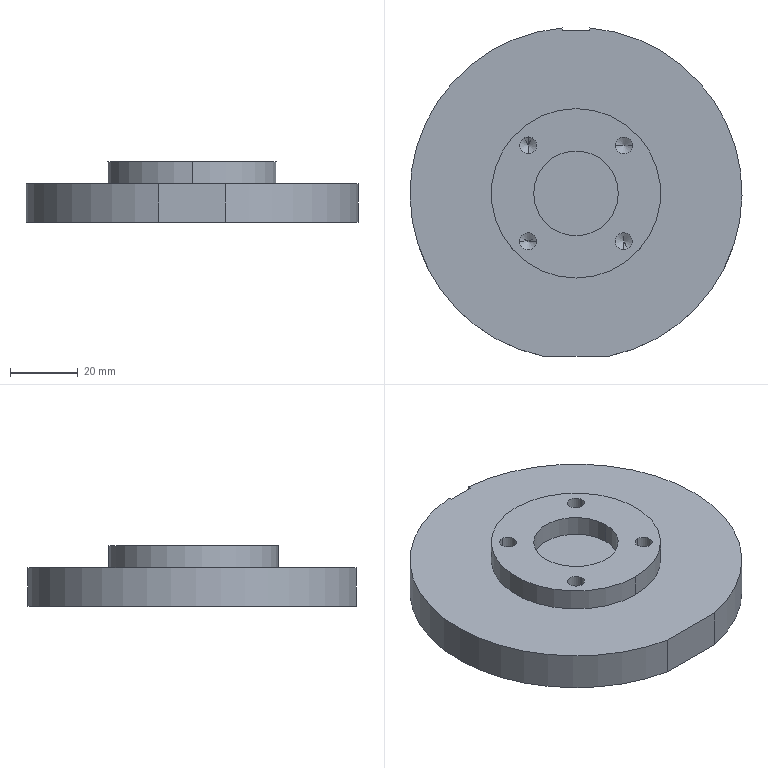Part | STEP file | Link6 | 1 solid | 30 faces | box 98 x 96.836 x 18 mm | volume 95263 mm3 | cylinder 14 | cone 8 | plane 8 | commonest cylinder face diameters 5 x8 25 x2 50 x2 98 x2
STEP:
#1=CARTESIAN_POINT('',(-12.5,0.,-6.));
#2=VERTEX_POINT('',#1);
#3=CARTESIAN_POINT('',(12.5,0.,-6.));
#4=VERTEX_POINT('',#3);
#5=CARTESIAN_POINT('',(0.,0.,-6.));
#6=DIRECTION('',(0.,0.,1.));
#7=DIRECTION('',(1.,0.,0.));
#8=AXIS2_PLACEMENT_3D('',#5,#6,#7);
#9=CIRCLE('',#8,12.5);
#10=EDGE_CURVE('',#2,#4,#9,.T.);
#11=ORIENTED_EDGE('',*,*,#10,.F.);
#12=CARTESIAN_POINT('',(-12.5,0.,0.));
#13=VERTEX_POINT('',#12);
#14=CARTESIAN_POINT('',(-12.5,0.,-6.));
#15=DIRECTION('',(0.,0.,1.));
#16=VECTOR('',#15,1000.);
#17=LINE('',#14,#16);
#18=EDGE_CURVE('',#2,#13,#17,.T.);
#19=ORIENTED_EDGE('',*,*,#18,.T.);
#20=CARTESIAN_POINT('',(12.5,0.,0.));
#21=VERTEX_POINT('',#20);
#22=CARTESIAN_POINT('',(0.,0.,0.));
#23=DIRECTION('',(0.,0.,1.));
#24=DIRECTION('',(1.,0.,0.));
#25=AXIS2_PLACEMENT_3D('',#22,#23,#24);
#26=CIRCLE('',#25,12.5);
#27=EDGE_CURVE('',#13,#21,#26,.T.);
#28=ORIENTED_EDGE('',*,*,#27,.T.);
#29=CARTESIAN_POINT('',(12.5,0.,-6.));
#30=DIRECTION('',(0.,0.,1.));
#31=VECTOR('',#30,1000.);
#32=LINE('',#29,#31);
#33=EDGE_CURVE('',#4,#21,#32,.T.);
#34=ORIENTED_EDGE('',*,*,#33,.F.);
#35=EDGE_LOOP('',(#11,#19,#28,#34));
#36=FACE_OUTER_BOUND('',#35,.T.);
#37=CARTESIAN_POINT('',(0.,0.,-6.));
#38=DIRECTION('',(0.,0.,1.));
#39=DIRECTION('',(1.,0.,0.));
#40=AXIS2_PLACEMENT_3D('',#37,#38,#39);
#41=CYLINDRICAL_SURFACE('',#40,12.5);
#42=ADVANCED_FACE('',(#36),#41,.F.);
#43=CARTESIAN_POINT('',(-14.142,11.642,-13.));
#44=VERTEX_POINT('',#43);
#45=CARTESIAN_POINT('',(-14.142,16.642,-13.));
#46=VERTEX_POINT('',#45);
#47=CARTESIAN_POINT('',(-14.142,14.142,-13.));
#48=DIRECTION('',(0.,0.,1.));
#49=DIRECTION('',(0.,1.,0.));
#50=AXIS2_PLACEMENT_3D('',#47,#48,#49);
#51=CIRCLE('',#50,2.5);
#52=EDGE_CURVE('',#44,#46,#51,.T.);
#53=ORIENTED_EDGE('',*,*,#52,.F.);
#54=CARTESIAN_POINT('',(-14.142,11.642,0.));
#55=VERTEX_POINT('',#54);
#56=CARTESIAN_POINT('',(-14.142,11.642,0.));
#57=DIRECTION('',(0.,0.,1.));
#58=VECTOR('',#57,1000.);
#59=LINE('',#56,#58);
#60=EDGE_CURVE('',#44,#55,#59,.T.);
#61=ORIENTED_EDGE('',*,*,#60,.T.);
#62=CARTESIAN_POINT('',(-14.142,16.642,0.));
#63=VERTEX_POINT('',#62);
#64=CARTESIAN_POINT('',(-14.142,14.142,0.));
#65=DIRECTION('',(0.,0.,1.));
#66=DIRECTION('',(0.,1.,0.));
#67=AXIS2_PLACEMENT_3D('',#64,#65,#66);
#68=CIRCLE('',#67,2.5);
#69=EDGE_CURVE('',#55,#63,#68,.T.);
#70=ORIENTED_EDGE('',*,*,#69,.T.);
#71=CARTESIAN_POINT('',(-14.142,16.642,0.));
#72=DIRECTION('',(0.,0.,1.));
#73=VECTOR('',#72,1000.);
#74=LINE('',#71,#73);
#75=EDGE_CURVE('',#46,#63,#74,.T.);
#76=ORIENTED_EDGE('',*,*,#75,.F.);
#77=EDGE_LOOP('',(#53,#61,#70,#76));
#78=FACE_OUTER_BOUND('',#77,.T.);
#79=CARTESIAN_POINT('',(-14.142,14.142,0.));
#80=DIRECTION('',(0.,0.,1.));
#81=DIRECTION('',(0.,1.,0.));
#82=AXIS2_PLACEMENT_3D('',#79,#80,#81);
#83=CYLINDRICAL_SURFACE('',#82,2.5);
#84=ADVANCED_FACE('',(#78),#83,.F.);
#85=CARTESIAN_POINT('',(-14.142,14.142,-14.502));
#86=VERTEX_POINT('',#85);
#87=CARTESIAN_POINT('',(-14.142,16.642,-13.));
#88=DIRECTION('',(0.,0.8572,0.515));
#89=VECTOR('',#88,1000.);
#90=LINE('',#87,#89);
#91=EDGE_CURVE('',#86,#46,#90,.T.);
#92=ORIENTED_EDGE('',*,*,#91,.F.);
#93=CARTESIAN_POINT('',(-14.142,11.642,-13.));
#94=DIRECTION('',(0.,-0.8572,0.515));
#95=VECTOR('',#94,1000.);
#96=LINE('',#93,#95);
#97=EDGE_CURVE('',#86,#44,#96,.T.);
#98=ORIENTED_EDGE('',*,*,#97,.T.);
#99=ORIENTED_EDGE('',*,*,#52,.T.);
#100=EDGE_LOOP('',(#92,#98,#99));
#101=FACE_OUTER_BOUND('',#100,.T.);
#102=CARTESIAN_POINT('',(-14.142,14.142,-13.));
#103=DIRECTION('',(0.,0.,1.));
#104=DIRECTION('',(0.,1.,0.));
#105=AXIS2_PLACEMENT_3D('',#102,#103,#104);
#106=CONICAL_SURFACE('',#105,2.5,1.03);
#107=ADVANCED_FACE('',(#101),#106,.F.);
#108=CARTESIAN_POINT('',(-11.642,-14.142,-13.));
#109=VERTEX_POINT('',#108);
#110=CARTESIAN_POINT('',(-16.642,-14.142,-13.));
#111=VERTEX_POINT('',#110);
#112=CARTESIAN_POINT('',(-14.142,-14.142,-13.));
#113=DIRECTION('',(0.,0.,1.));
#114=DIRECTION('',(-1.,0.,0.));
#115=AXIS2_PLACEMENT_3D('',#112,#113,#114);
#116=CIRCLE('',#115,2.5);
#117=EDGE_CURVE('',#109,#111,#116,.T.);
#118=ORIENTED_EDGE('',*,*,#117,.F.);
#119=CARTESIAN_POINT('',(-11.642,-14.142,0.));
#120=VERTEX_POINT('',#119);
#121=CARTESIAN_POINT('',(-11.642,-14.142,0.));
#122=DIRECTION('',(0.,0.,1.));
#123=VECTOR('',#122,1000.);
#124=LINE('',#121,#123);
#125=EDGE_CURVE('',#109,#120,#124,.T.);
#126=ORIENTED_EDGE('',*,*,#125,.T.);
#127=CARTESIAN_POINT('',(-16.642,-14.142,0.));
#128=VERTEX_POINT('',#127);
#129=CARTESIAN_POINT('',(-14.142,-14.142,0.));
#130=DIRECTION('',(0.,0.,1.));
#131=DIRECTION('',(-1.,0.,0.));
#132=AXIS2_PLACEMENT_3D('',#129,#130,#131);
#133=CIRCLE('',#132,2.5);
#134=EDGE_CURVE('',#120,#128,#133,.T.);
#135=ORIENTED_EDGE('',*,*,#134,.T.);
#136=CARTESIAN_POINT('',(-16.642,-14.142,0.));
#137=DIRECTION('',(0.,0.,1.));
#138=VECTOR('',#137,1000.);
#139=LINE('',#136,#138);
#140=EDGE_CURVE('',#111,#128,#139,.T.);
#141=ORIENTED_EDGE('',*,*,#140,.F.);
#142=EDGE_LOOP('',(#118,#126,#135,#141));
#143=FACE_OUTER_BOUND('',#142,.T.);
#144=CARTESIAN_POINT('',(-14.142,-14.142,0.));
#145=DIRECTION('',(0.,0.,1.));
#146=DIRECTION('',(-1.,0.,0.));
#147=AXIS2_PLACEMENT_3D('',#144,#145,#146);
#148=CYLINDRICAL_SURFACE('',#147,2.5);
#149=ADVANCED_FACE('',(#143),#148,.F.);
#150=CARTESIAN_POINT('',(-14.142,-14.142,-14.502));
#151=VERTEX_POINT('',#150);
#152=CARTESIAN_POINT('',(-16.642,-14.142,-13.));
#153=DIRECTION('',(-0.8572,0.,0.515));
#154=VECTOR('',#153,1000.);
#155=LINE('',#152,#154);
#156=EDGE_CURVE('',#151,#111,#155,.T.);
#157=ORIENTED_EDGE('',*,*,#156,.F.);
#158=CARTESIAN_POINT('',(-11.642,-14.142,-13.));
#159=DIRECTION('',(0.8572,0.,0.515));
#160=VECTOR('',#159,1000.);
#161=LINE('',#158,#160);
#162=EDGE_CURVE('',#151,#109,#161,.T.);
#163=ORIENTED_EDGE('',*,*,#162,.T.);
#164=ORIENTED_EDGE('',*,*,#117,.T.);
#165=EDGE_LOOP('',(#157,#163,#164));
#166=FACE_OUTER_BOUND('',#165,.T.);
#167=CARTESIAN_POINT('',(-14.142,-14.142,-13.));
#168=DIRECTION('',(0.,0.,1.));
#169=DIRECTION('',(-1.,0.,0.));
#170=AXIS2_PLACEMENT_3D('',#167,#168,#169);
#171=CONICAL_SURFACE('',#170,2.5,1.03);
#172=ADVANCED_FACE('',(#166),#171,.F.);
#173=CARTESIAN_POINT('',(14.142,-11.642,-13.));
#174=VERTEX_POINT('',#173);
#175=CARTESIAN_POINT('',(14.142,-16.642,-13.));
#176=VERTEX_POINT('',#175);
#177=CARTESIAN_POINT('',(14.142,-14.142,-13.));
#178=DIRECTION('',(0.,0.,1.));
#179=DIRECTION('',(0.,-1.,0.));
#180=AXIS2_PLACEMENT_3D('',#177,#178,#179);
#181=CIRCLE('',#180,2.5);
#182=EDGE_CURVE('',#174,#176,#181,.T.);
#183=ORIENTED_EDGE('',*,*,#182,.F.);
#184=CARTESIAN_POINT('',(14.142,-11.642,0.));
#185=VERTEX_POINT('',#184);
#186=CARTESIAN_POINT('',(14.142,-11.642,0.));
#187=DIRECTION('',(0.,0.,1.));
#188=VECTOR('',#187,1000.);
#189=LINE('',#186,#188);
#190=EDGE_CURVE('',#174,#185,#189,.T.);
#191=ORIENTED_EDGE('',*,*,#190,.T.);
#192=CARTESIAN_POINT('',(14.142,-16.642,0.));
#193=VERTEX_POINT('',#192);
#194=CARTESIAN_POINT('',(14.142,-14.142,0.));
#195=DIRECTION('',(0.,0.,1.));
#196=DIRECTION('',(0.,-1.,0.));
#197=AXIS2_PLACEMENT_3D('',#194,#195,#196);
#198=CIRCLE('',#197,2.5);
#199=EDGE_CURVE('',#185,#193,#198,.T.);
#200=ORIENTED_EDGE('',*,*,#199,.T.);
#201=CARTESIAN_POINT('',(14.142,-16.642,0.));
#202=DIRECTION('',(0.,0.,1.));
#203=VECTOR('',#202,1000.);
#204=LINE('',#201,#203);
#205=EDGE_CURVE('',#176,#193,#204,.T.);
#206=ORIENTED_EDGE('',*,*,#205,.F.);
#207=EDGE_LOOP('',(#183,#191,#200,#206));
#208=FACE_OUTER_BOUND('',#207,.T.);
#209=CARTESIAN_POINT('',(14.142,-14.142,0.));
#210=DIRECTION('',(0.,0.,1.));
#211=DIRECTION('',(0.,-1.,0.));
#212=AXIS2_PLACEMENT_3D('',#209,#210,#211);
#213=CYLINDRICAL_SURFACE('',#212,2.5);
#214=ADVANCED_FACE('',(#208),#213,.F.);
#215=CARTESIAN_POINT('',(14.142,-14.142,-14.502));
#216=VERTEX_POINT('',#215);
#217=CARTESIAN_POINT('',(14.142,-16.642,-13.));
#218=DIRECTION('',(0.,-0.8572,0.515));
#219=VECTOR('',#218,1000.);
#220=LINE('',#217,#219);
#221=EDGE_CURVE('',#216,#176,#220,.T.);
#222=ORIENTED_EDGE('',*,*,#221,.F.);
#223=CARTESIAN_POINT('',(14.142,-11.642,-13.));
#224=DIRECTION('',(0.,0.8572,0.515));
#225=VECTOR('',#224,1000.);
#226=LINE('',#223,#225);
#227=EDGE_CURVE('',#216,#174,#226,.T.);
#228=ORIENTED_EDGE('',*,*,#227,.T.);
#229=ORIENTED_EDGE('',*,*,#182,.T.);
#230=EDGE_LOOP('',(#222,#228,#229));
#231=FACE_OUTER_BOUND('',#230,.T.);
#232=CARTESIAN_POINT('',(14.142,-14.142,-13.));
#233=DIRECTION('',(0.,0.,1.));
#234=DIRECTION('',(0.,-1.,0.));
#235=AXIS2_PLACEMENT_3D('',#232,#233,#234);
#236=CONICAL_SURFACE('',#235,2.5,1.03);
#237=ADVANCED_FACE('',(#231),#236,.F.);
#238=CARTESIAN_POINT('',(11.642,14.142,-13.));
#239=VERTEX_POINT('',#238);
#240=CARTESIAN_POINT('',(16.642,14.142,-13.));
#241=VERTEX_POINT('',#240);
#242=CARTESIAN_POINT('',(14.142,14.142,-13.));
#243=DIRECTION('',(0.,0.,1.));
#244=DIRECTION('',(1.,0.,0.));
#245=AXIS2_PLACEMENT_3D('',#242,#243,#244);
#246=CIRCLE('',#245,2.5);
#247=EDGE_CURVE('',#239,#241,#246,.T.);
#248=ORIENTED_EDGE('',*,*,#247,.F.);
#249=CARTESIAN_POINT('',(11.642,14.142,0.));
#250=VERTEX_POINT('',#249);
#251=CARTESIAN_POINT('',(11.642,14.142,0.));
#252=DIRECTION('',(0.,0.,1.));
#253=VECTOR('',#252,1000.);
#254=LINE('',#251,#253);
#255=EDGE_CURVE('',#239,#250,#254,.T.);
#256=ORIENTED_EDGE('',*,*,#255,.T.);
#257=CARTESIAN_POINT('',(16.642,14.142,0.));
#258=VERTEX_POINT('',#257);
#259=CARTESIAN_POINT('',(14.142,14.142,0.));
#260=DIRECTION('',(0.,0.,1.));
#261=DIRECTION('',(1.,0.,0.));
#262=AXIS2_PLACEMENT_3D('',#259,#260,#261);
#263=CIRCLE('',#262,2.5);
#264=EDGE_CURVE('',#250,#258,#263,.T.);
#265=ORIENTED_EDGE('',*,*,#264,.T.);
#266=CARTESIAN_POINT('',(16.642,14.142,0.));
#267=DIRECTION('',(0.,0.,1.));
#268=VECTOR('',#267,1000.);
#269=LINE('',#266,#268);
#270=EDGE_CURVE('',#241,#258,#269,.T.);
#271=ORIENTED_EDGE('',*,*,#270,.F.);
#272=EDGE_LOOP('',(#248,#256,#265,#271));
#273=FACE_OUTER_BOUND('',#272,.T.);
#274=CARTESIAN_POINT('',(14.142,14.142,0.));
#275=DIRECTION('',(0.,0.,1.));
#276=DIRECTION('',(1.,0.,0.));
#277=AXIS2_PLACEMENT_3D('',#274,#275,#276);
#278=CYLINDRICAL_SURFACE('',#277,2.5);
#279=ADVANCED_FACE('',(#273),#278,.F.);
#280=CARTESIAN_POINT('',(14.142,14.142,-14.502));
#281=VERTEX_POINT('',#280);
#282=CARTESIAN_POINT('',(16.642,14.142,-13.));
#283=DIRECTION('',(0.8572,0.,0.515));
#284=VECTOR('',#283,1000.);
#285=LINE('',#282,#284);
#286=EDGE_CURVE('',#281,#241,#285,.T.);
#287=ORIENTED_EDGE('',*,*,#286,.F.);
#288=CARTESIAN_POINT('',(11.642,14.142,-13.));
#289=DIRECTION('',(-0.8572,0.,0.515));
#290=VECTOR('',#289,1000.);
#291=LINE('',#288,#290);
#292=EDGE_CURVE('',#281,#239,#291,.T.);
#293=ORIENTED_EDGE('',*,*,#292,.T.);
#294=ORIENTED_EDGE('',*,*,#247,.T.);
#295=EDGE_LOOP('',(#287,#293,#294));
#296=FACE_OUTER_BOUND('',#295,.T.);
#297=CARTESIAN_POINT('',(14.142,14.142,-13.));
#298=DIRECTION('',(0.,0.,1.));
#299=DIRECTION('',(1.,0.,0.));
#300=AXIS2_PLACEMENT_3D('',#297,#298,#299);
#301=CONICAL_SURFACE('',#300,2.5,1.03);
#302=ADVANCED_FACE('',(#296),#301,.F.);
#303=CARTESIAN_POINT('',(0.,25.,0.));
#304=VERTEX_POINT('',#303);
#305=CARTESIAN_POINT('',(0.,-25.,0.));
#306=VERTEX_POINT('',#305);
#307=CARTESIAN_POINT('',(0.,0.,0.));
#308=DIRECTION('',(0.,0.,-1.));
#309=DIRECTION('',(0.,1.,0.));
#310=AXIS2_PLACEMENT_3D('',#307,#308,#309);
#311=CIRCLE('',#310,25.);
#312=EDGE_CURVE('',#304,#306,#311,.T.);
#313=ORIENTED_EDGE('',*,*,#312,.T.);
#314=CARTESIAN_POINT('',(0.,-25.,-6.5));
#315=VERTEX_POINT('',#314);
#316=CARTESIAN_POINT('',(0.,-25.,-3.25));
#317=DIRECTION('',(0.,0.,-1.));
#318=VECTOR('',#317,1000.);
#319=LINE('',#316,#318);
#320=EDGE_CURVE('',#306,#315,#319,.T.);
#321=ORIENTED_EDGE('',*,*,#320,.T.);
#322=CARTESIAN_POINT('',(0.,25.,-6.5));
#323=VERTEX_POINT('',#322);
#324=CARTESIAN_POINT('',(0.,0.,-6.5));
#325=DIRECTION('',(0.,0.,-1.));
#326=DIRECTION('',(0.,1.,0.));
#327=AXIS2_PLACEMENT_3D('',#324,#325,#326);
#328=CIRCLE('',#327,25.);
#329=EDGE_CURVE('',#323,#315,#328,.T.);
#330=ORIENTED_EDGE('',*,*,#329,.F.);
#331=CARTESIAN_POINT('',(0.,25.,-3.25));
#332=DIRECTION('',(0.,0.,-1.));
#333=VECTOR('',#332,1000.);
#334=LINE('',#331,#333);
#335=EDGE_CURVE('',#304,#323,#334,.T.);
#336=ORIENTED_EDGE('',*,*,#335,.F.);
#337=EDGE_LOOP('',(#313,#321,#330,#336));
#338=FACE_OUTER_BOUND('',#337,.T.);
#339=CARTESIAN_POINT('',(0.,0.,-3.25));
#340=DIRECTION('',(0.,0.,-1.));
#341=DIRECTION('',(0.,1.,0.));
#342=AXIS2_PLACEMENT_3D('',#339,#340,#341);
#343=CYLINDRICAL_SURFACE('',#342,25.);
#344=ADVANCED_FACE('',(#338),#343,.T.);
#345=CARTESIAN_POINT('',(4.,48.,-18.));
#346=VERTEX_POINT('',#345);
#347=CARTESIAN_POINT('',(4.,48.836,-18.));
#348=VERTEX_POINT('',#347);
#349=CARTESIAN_POINT('',(4.,48.836,-18.));
#350=DIRECTION('',(0.,1.,0.));
#351=VECTOR('',#350,1000.);
#352=LINE('',#349,#351);
#353=EDGE_CURVE('',#346,#348,#352,.T.);
#354=ORIENTED_EDGE('',*,*,#353,.T.);
#355=CARTESIAN_POINT('',(9.849,-48.,-18.));
#356=VERTEX_POINT('',#355);
#357=CARTESIAN_POINT('',(0.,0.,-18.));
#358=DIRECTION('',(0.,0.,-1.));
#359=DIRECTION('',(0.,1.,0.));
#360=AXIS2_PLACEMENT_3D('',#357,#358,#359);
#361=CIRCLE('',#360,49.);
#362=EDGE_CURVE('',#348,#356,#361,.T.);
#363=ORIENTED_EDGE('',*,*,#362,.T.);
#364=CARTESIAN_POINT('',(-9.849,-48.,-18.));
#365=VERTEX_POINT('',#364);
#366=CARTESIAN_POINT('',(0.,-48.,-18.));
#367=DIRECTION('',(-1.,0.,0.));
#368=VECTOR('',#367,1000.);
#369=LINE('',#366,#368);
#370=EDGE_CURVE('',#356,#365,#369,.T.);
#371=ORIENTED_EDGE('',*,*,#370,.T.);
#372=CARTESIAN_POINT('',(-4.,48.836,-18.));
#373=VERTEX_POINT('',#372);
#374=CARTESIAN_POINT('',(0.,0.,-18.));
#375=DIRECTION('',(0.,0.,-1.));
#376=DIRECTION('',(0.,1.,0.));
#377=AXIS2_PLACEMENT_3D('',#374,#375,#376);
#378=CIRCLE('',#377,49.);
#379=EDGE_CURVE('',#365,#373,#378,.T.);
#380=ORIENTED_EDGE('',*,*,#379,.T.);
#381=CARTESIAN_POINT('',(-4.,48.,-18.));
#382=VERTEX_POINT('',#381);
#383=CARTESIAN_POINT('',(-4.,48.,-18.));
#384=DIRECTION('',(0.,-1.,0.));
#385=VECTOR('',#384,1000.);
#386=LINE('',#383,#385);
#387=EDGE_CURVE('',#373,#382,#386,.T.);
#388=ORIENTED_EDGE('',*,*,#387,.T.);
#389=CARTESIAN_POINT('',(0.,48.,-18.));
#390=DIRECTION('',(1.,0.,0.));
#391=VECTOR('',#390,1000.);
#392=LINE('',#389,#391);
#393=EDGE_CURVE('',#382,#346,#392,.T.);
#394=ORIENTED_EDGE('',*,*,#393,.T.);
#395=EDGE_LOOP('',(#354,#363,#371,#380,#388,#394));
#396=FACE_OUTER_BOUND('',#395,.T.);
#397=CARTESIAN_POINT('',(0.,24.5,-18.));
#398=DIRECTION('',(0.,0.,-1.));
#399=DIRECTION('',(-1.,0.,0.));
#400=AXIS2_PLACEMENT_3D('',#397,#398,#399);
#401=PLANE('',#400);
#402=ADVANCED_FACE('',(#396),#401,.T.);
#403=CARTESIAN_POINT('',(4.,48.836,-6.5));
#404=VERTEX_POINT('',#403);
#405=CARTESIAN_POINT('',(4.,48.836,-12.25));
#406=DIRECTION('',(0.,0.,1.));
#407=VECTOR('',#406,1000.);
#408=LINE('',#405,#407);
#409=EDGE_CURVE('',#348,#404,#408,.T.);
#410=ORIENTED_EDGE('',*,*,#409,.T.);
#411=CARTESIAN_POINT('',(9.849,-48.,-6.5));
#412=VERTEX_POINT('',#411);
#413=CARTESIAN_POINT('',(0.,0.,-6.5));
#414=DIRECTION('',(0.,0.,-1.));
#415=DIRECTION('',(0.,1.,0.));
#416=AXIS2_PLACEMENT_3D('',#413,#414,#415);
#417=CIRCLE('',#416,49.);
#418=EDGE_CURVE('',#404,#412,#417,.T.);
#419=ORIENTED_EDGE('',*,*,#418,.T.);
#420=CARTESIAN_POINT('',(9.849,-48.,-12.25));
#421=DIRECTION('',(0.,0.,-1.));
#422=VECTOR('',#421,1000.);
#423=LINE('',#420,#422);
#424=EDGE_CURVE('',#412,#356,#423,.T.);
#425=ORIENTED_EDGE('',*,*,#424,.T.);
#426=ORIENTED_EDGE('',*,*,#362,.F.);
#427=EDGE_LOOP('',(#410,#419,#425,#426));
#428=FACE_OUTER_BOUND('',#427,.T.);
#429=CARTESIAN_POINT('',(0.,0.,-12.25));
#430=DIRECTION('',(0.,0.,-1.));
#431=DIRECTION('',(0.,1.,0.));
#432=AXIS2_PLACEMENT_3D('',#429,#430,#431);
#433=CYLINDRICAL_SURFACE('',#432,49.);
#434=ADVANCED_FACE('',(#428),#433,.T.);
#435=CARTESIAN_POINT('',(4.,48.,-6.5));
#436=VERTEX_POINT('',#435);
#437=CARTESIAN_POINT('',(4.,48.,-18.));
#438=DIRECTION('',(0.,0.,1.));
#439=VECTOR('',#438,1000.);
#440=LINE('',#437,#439);
#441=EDGE_CURVE('',#346,#436,#440,.T.);
#442=ORIENTED_EDGE('',*,*,#441,.F.);
#443=ORIENTED_EDGE('',*,*,#393,.F.);
#444=CARTESIAN_POINT('',(-4.,48.,-6.5));
#445=VERTEX_POINT('',#444);
#446=CARTESIAN_POINT('',(-4.,48.,-18.));
#447=DIRECTION('',(0.,0.,-1.));
#448=VECTOR('',#447,1000.);
#449=LINE('',#446,#448);
#450=EDGE_CURVE('',#445,#382,#449,.T.);
#451=ORIENTED_EDGE('',*,*,#450,.F.);
#452=CARTESIAN_POINT('',(4.,48.,-6.5));
#453=DIRECTION('',(-1.,0.,0.));
#454=VECTOR('',#453,1000.);
#455=LINE('',#452,#454);
#456=EDGE_CURVE('',#436,#445,#455,.T.);
#457=ORIENTED_EDGE('',*,*,#456,.F.);
#458=EDGE_LOOP('',(#442,#443,#451,#457));
#459=FACE_OUTER_BOUND('',#458,.T.);
#460=CARTESIAN_POINT('',(4.,48.,-18.));
#461=DIRECTION('',(0.,-1.,0.));
#462=DIRECTION('',(0.,0.,-1.));
#463=AXIS2_PLACEMENT_3D('',#460,#461,#462);
#464=PLANE('',#463);
#465=ADVANCED_FACE('',(#459),#464,.F.);
#466=CARTESIAN_POINT('',(-4.,48.836,-6.5));
#467=VERTEX_POINT('',#466);
#468=CARTESIAN_POINT('',(-4.,48.836,-12.25));
#469=DIRECTION('',(0.,0.,-1.));
#470=VECTOR('',#469,1000.);
#471=LINE('',#468,#470);
#472=EDGE_CURVE('',#467,#373,#471,.T.);
#473=ORIENTED_EDGE('',*,*,#472,.T.);
#474=ORIENTED_EDGE('',*,*,#379,.F.);
#475=CARTESIAN_POINT('',(-9.849,-48.,-6.5));
#476=VERTEX_POINT('',#475);
#477=CARTESIAN_POINT('',(-9.849,-48.,-12.25));
#478=DIRECTION('',(0.,0.,1.));
#479=VECTOR('',#478,1000.);
#480=LINE('',#477,#479);
#481=EDGE_CURVE('',#365,#476,#480,.T.);
#482=ORIENTED_EDGE('',*,*,#481,.T.);
#483=CARTESIAN_POINT('',(0.,0.,-6.5));
#484=DIRECTION('',(0.,0.,-1.));
#485=DIRECTION('',(0.,1.,0.));
#486=AXIS2_PLACEMENT_3D('',#483,#484,#485);
#487=CIRCLE('',#486,49.);
#488=EDGE_CURVE('',#476,#467,#487,.T.);
#489=ORIENTED_EDGE('',*,*,#488,.T.);
#490=EDGE_LOOP('',(#473,#474,#482,#489));
#491=FACE_OUTER_BOUND('',#490,.T.);
#492=CARTESIAN_POINT('',(0.,0.,-12.25));
#493=DIRECTION('',(0.,0.,-1.));
#494=DIRECTION('',(0.,1.,0.));
#495=AXIS2_PLACEMENT_3D('',#492,#493,#494);
#496=CYLINDRICAL_SURFACE('',#495,49.);
#497=ADVANCED_FACE('',(#491),#496,.T.);
#498=ORIENTED_EDGE('',*,*,#481,.F.);
#499=ORIENTED_EDGE('',*,*,#370,.F.);
#500=ORIENTED_EDGE('',*,*,#424,.F.);
#501=CARTESIAN_POINT('',(-9.849,-48.,-6.5));
#502=DIRECTION('',(1.,0.,0.));
#503=VECTOR('',#502,1000.);
#504=LINE('',#501,#503);
#505=EDGE_CURVE('',#476,#412,#504,.T.);
#506=ORIENTED_EDGE('',*,*,#505,.F.);
#507=EDGE_LOOP('',(#498,#499,#500,#506));
#508=FACE_OUTER_BOUND('',#507,.T.);
#509=CARTESIAN_POINT('',(-9.849,-48.,-18.));
#510=DIRECTION('',(0.,1.,0.));
#511=DIRECTION('',(0.,0.,1.));
#512=AXIS2_PLACEMENT_3D('',#509,#510,#511);
#513=PLANE('',#512);
#514=ADVANCED_FACE('',(#508),#513,.F.);
#515=ORIENTED_EDGE('',*,*,#329,.T.);
#516=CARTESIAN_POINT('',(0.,0.,-6.5));
#517=DIRECTION('',(0.,0.,-1.));
#518=DIRECTION('',(0.,1.,0.));
#519=AXIS2_PLACEMENT_3D('',#516,#517,#518);
#520=CIRCLE('',#519,25.);
#521=EDGE_CURVE('',#315,#323,#520,.T.);
#522=ORIENTED_EDGE('',*,*,#521,.T.);
#523=EDGE_LOOP('',(#515,#522));
#524=FACE_BOUND('',#523,.T.);
#525=CARTESIAN_POINT('',(-4.,37.,-6.5));
#526=DIRECTION('',(0.,1.,0.));
#527=VECTOR('',#526,1000.);
#528=LINE('',#525,#527);
#529=EDGE_CURVE('',#445,#467,#528,.T.);
#530=ORIENTED_EDGE('',*,*,#529,.T.);
#531=ORIENTED_EDGE('',*,*,#488,.F.);
#532=ORIENTED_EDGE('',*,*,#505,.T.);
#533=ORIENTED_EDGE('',*,*,#418,.F.);
#534=CARTESIAN_POINT('',(4.,37.,-6.5));
#535=DIRECTION('',(0.,-1.,0.));
#536=VECTOR('',#535,1000.);
#537=LINE('',#534,#536);
#538=EDGE_CURVE('',#404,#436,#537,.T.);
#539=ORIENTED_EDGE('',*,*,#538,.T.);
#540=ORIENTED_EDGE('',*,*,#456,.T.);
#541=EDGE_LOOP('',(#530,#531,#532,#533,#539,#540));
#542=FACE_OUTER_BOUND('',#541,.T.);
#543=CARTESIAN_POINT('',(0.,37.,-6.5));
#544=DIRECTION('',(0.,0.,1.));
#545=DIRECTION('',(1.,0.,0.));
#546=AXIS2_PLACEMENT_3D('',#543,#544,#545);
#547=PLANE('',#546);
#548=ADVANCED_FACE('',(#524,#542),#547,.T.);
#549=ORIENTED_EDGE('',*,*,#409,.F.);
#550=ORIENTED_EDGE('',*,*,#353,.F.);
#551=ORIENTED_EDGE('',*,*,#441,.T.);
#552=ORIENTED_EDGE('',*,*,#538,.F.);
#553=EDGE_LOOP('',(#549,#550,#551,#552));
#554=FACE_OUTER_BOUND('',#553,.T.);
#555=CARTESIAN_POINT('',(4.,48.836,-18.));
#556=DIRECTION('',(1.,0.,0.));
#557=DIRECTION('',(0.,0.,-1.));
#558=AXIS2_PLACEMENT_3D('',#555,#556,#557);
#559=PLANE('',#558);
#560=ADVANCED_FACE('',(#554),#559,.F.);
#561=ORIENTED_EDGE('',*,*,#450,.T.);
#562=ORIENTED_EDGE('',*,*,#387,.F.);
#563=ORIENTED_EDGE('',*,*,#472,.F.);
#564=ORIENTED_EDGE('',*,*,#529,.F.);
#565=EDGE_LOOP('',(#561,#562,#563,#564));
#566=FACE_OUTER_BOUND('',#565,.T.);
#567=CARTESIAN_POINT('',(-4.,48.,-18.));
#568=DIRECTION('',(-1.,0.,0.));
#569=DIRECTION('',(0.,0.,1.));
#570=AXIS2_PLACEMENT_3D('',#567,#568,#569);
#571=PLANE('',#570);
#572=ADVANCED_FACE('',(#566),#571,.F.);
#573=ORIENTED_EDGE('',*,*,#320,.F.);
#574=CARTESIAN_POINT('',(0.,0.,0.));
#575=DIRECTION('',(0.,0.,-1.));
#576=DIRECTION('',(0.,1.,0.));
#577=AXIS2_PLACEMENT_3D('',#574,#575,#576);
#578=CIRCLE('',#577,25.);
#579=EDGE_CURVE('',#306,#304,#578,.T.);
#580=ORIENTED_EDGE('',*,*,#579,.T.);
#581=ORIENTED_EDGE('',*,*,#335,.T.);
#582=ORIENTED_EDGE('',*,*,#521,.F.);
#583=EDGE_LOOP('',(#573,#580,#581,#582));
#584=FACE_OUTER_BOUND('',#583,.T.);
#585=CARTESIAN_POINT('',(0.,0.,-3.25));
#586=DIRECTION('',(0.,0.,-1.));
#587=DIRECTION('',(0.,1.,0.));
#588=AXIS2_PLACEMENT_3D('',#585,#586,#587);
#589=CYLINDRICAL_SURFACE('',#588,25.);
#590=ADVANCED_FACE('',(#584),#589,.T.);
#591=CARTESIAN_POINT('',(0.,0.,0.));
#592=DIRECTION('',(0.,0.,1.));
#593=DIRECTION('',(1.,0.,0.));
#594=AXIS2_PLACEMENT_3D('',#591,#592,#593);
#595=CIRCLE('',#594,12.5);
#596=EDGE_CURVE('',#21,#13,#595,.T.);
#597=ORIENTED_EDGE('',*,*,#596,.F.);
#598=ORIENTED_EDGE('',*,*,#27,.F.);
#599=EDGE_LOOP('',(#597,#598));
#600=FACE_BOUND('',#599,.T.);
#601=CARTESIAN_POINT('',(-14.142,14.142,0.));
#602=DIRECTION('',(0.,0.,1.));
#603=DIRECTION('',(0.,1.,0.));
#604=AXIS2_PLACEMENT_3D('',#601,#602,#603);
#605=CIRCLE('',#604,2.5);
#606=EDGE_CURVE('',#63,#55,#605,.T.);
#607=ORIENTED_EDGE('',*,*,#606,.F.);
#608=ORIENTED_EDGE('',*,*,#69,.F.);
#609=EDGE_LOOP('',(#607,#608));
#610=FACE_BOUND('',#609,.T.);
#611=CARTESIAN_POINT('',(-14.142,-14.142,0.));
#612=DIRECTION('',(0.,0.,1.));
#613=DIRECTION('',(-1.,0.,0.));
#614=AXIS2_PLACEMENT_3D('',#611,#612,#613);
#615=CIRCLE('',#614,2.5);
#616=EDGE_CURVE('',#128,#120,#615,.T.);
#617=ORIENTED_EDGE('',*,*,#616,.F.);
#618=ORIENTED_EDGE('',*,*,#134,.F.);
#619=EDGE_LOOP('',(#617,#618));
#620=FACE_BOUND('',#619,.T.);
#621=CARTESIAN_POINT('',(14.142,-14.142,0.));
#622=DIRECTION('',(0.,0.,1.));
#623=DIRECTION('',(0.,-1.,0.));
#624=AXIS2_PLACEMENT_3D('',#621,#622,#623);
#625=CIRCLE('',#624,2.5);
#626=EDGE_CURVE('',#193,#185,#625,.T.);
#627=ORIENTED_EDGE('',*,*,#626,.F.);
#628=ORIENTED_EDGE('',*,*,#199,.F.);
#629=EDGE_LOOP('',(#627,#628));
#630=FACE_BOUND('',#629,.T.);
#631=CARTESIAN_POINT('',(14.142,14.142,0.));
#632=DIRECTION('',(0.,0.,1.));
#633=DIRECTION('',(1.,0.,0.));
#634=AXIS2_PLACEMENT_3D('',#631,#632,#633);
#635=CIRCLE('',#634,2.5);
#636=EDGE_CURVE('',#258,#250,#635,.T.);
#637=ORIENTED_EDGE('',*,*,#636,.F.);
#638=ORIENTED_EDGE('',*,*,#264,.F.);
#639=EDGE_LOOP('',(#637,#638));
#640=FACE_BOUND('',#639,.T.);
#641=ORIENTED_EDGE('',*,*,#312,.F.);
#642=ORIENTED_EDGE('',*,*,#579,.F.);
#643=EDGE_LOOP('',(#641,#642));
#644=FACE_OUTER_BOUND('',#643,.T.);
#645=CARTESIAN_POINT('',(0.,12.5,0.));
#646=DIRECTION('',(0.,0.,1.));
#647=DIRECTION('',(1.,0.,0.));
#648=AXIS2_PLACEMENT_3D('',#645,#646,#647);
#649=PLANE('',#648);
#650=ADVANCED_FACE('',(#600,#610,#620,#630,#640,#644),#649,.T.);
#651=ORIENTED_EDGE('',*,*,#292,.F.);
#652=ORIENTED_EDGE('',*,*,#286,.T.);
#653=CARTESIAN_POINT('',(14.142,14.142,-13.));
#654=DIRECTION('',(0.,0.,1.));
#655=DIRECTION('',(1.,0.,0.));
#656=AXIS2_PLACEMENT_3D('',#653,#654,#655);
#657=CIRCLE('',#656,2.5);
#658=EDGE_CURVE('',#241,#239,#657,.T.);
#659=ORIENTED_EDGE('',*,*,#658,.T.);
#660=EDGE_LOOP('',(#651,#652,#659));
#661=FACE_OUTER_BOUND('',#660,.T.);
#662=CARTESIAN_POINT('',(14.142,14.142,-13.));
#663=DIRECTION('',(0.,0.,1.));
#664=DIRECTION('',(1.,0.,0.));
#665=AXIS2_PLACEMENT_3D('',#662,#663,#664);
#666=CONICAL_SURFACE('',#665,2.5,1.03);
#667=ADVANCED_FACE('',(#661),#666,.F.);
#668=ORIENTED_EDGE('',*,*,#255,.F.);
#669=ORIENTED_EDGE('',*,*,#658,.F.);
#670=ORIENTED_EDGE('',*,*,#270,.T.);
#671=ORIENTED_EDGE('',*,*,#636,.T.);
#672=EDGE_LOOP('',(#668,#669,#670,#671));
#673=FACE_OUTER_BOUND('',#672,.T.);
#674=CARTESIAN_POINT('',(14.142,14.142,0.));
#675=DIRECTION('',(0.,0.,1.));
#676=DIRECTION('',(1.,0.,0.));
#677=AXIS2_PLACEMENT_3D('',#674,#675,#676);
#678=CYLINDRICAL_SURFACE('',#677,2.5);
#679=ADVANCED_FACE('',(#673),#678,.F.);
#680=ORIENTED_EDGE('',*,*,#227,.F.);
#681=ORIENTED_EDGE('',*,*,#221,.T.);
#682=CARTESIAN_POINT('',(14.142,-14.142,-13.));
#683=DIRECTION('',(0.,0.,1.));
#684=DIRECTION('',(0.,-1.,0.));
#685=AXIS2_PLACEMENT_3D('',#682,#683,#684);
#686=CIRCLE('',#685,2.5);
#687=EDGE_CURVE('',#176,#174,#686,.T.);
#688=ORIENTED_EDGE('',*,*,#687,.T.);
#689=EDGE_LOOP('',(#680,#681,#688));
#690=FACE_OUTER_BOUND('',#689,.T.);
#691=CARTESIAN_POINT('',(14.142,-14.142,-13.));
#692=DIRECTION('',(0.,0.,1.));
#693=DIRECTION('',(0.,-1.,0.));
#694=AXIS2_PLACEMENT_3D('',#691,#692,#693);
#695=CONICAL_SURFACE('',#694,2.5,1.03);
#696=ADVANCED_FACE('',(#690),#695,.F.);
#697=ORIENTED_EDGE('',*,*,#190,.F.);
#698=ORIENTED_EDGE('',*,*,#687,.F.);
#699=ORIENTED_EDGE('',*,*,#205,.T.);
#700=ORIENTED_EDGE('',*,*,#626,.T.);
#701=EDGE_LOOP('',(#697,#698,#699,#700));
#702=FACE_OUTER_BOUND('',#701,.T.);
#703=CARTESIAN_POINT('',(14.142,-14.142,0.));
#704=DIRECTION('',(0.,0.,1.));
#705=DIRECTION('',(0.,-1.,0.));
#706=AXIS2_PLACEMENT_3D('',#703,#704,#705);
#707=CYLINDRICAL_SURFACE('',#706,2.5);
#708=ADVANCED_FACE('',(#702),#707,.F.);
#709=ORIENTED_EDGE('',*,*,#162,.F.);
#710=ORIENTED_EDGE('',*,*,#156,.T.);
#711=CARTESIAN_POINT('',(-14.142,-14.142,-13.));
#712=DIRECTION('',(0.,0.,1.));
#713=DIRECTION('',(-1.,0.,0.));
#714=AXIS2_PLACEMENT_3D('',#711,#712,#713);
#715=CIRCLE('',#714,2.5);
#716=EDGE_CURVE('',#111,#109,#715,.T.);
#717=ORIENTED_EDGE('',*,*,#716,.T.);
#718=EDGE_LOOP('',(#709,#710,#717));
#719=FACE_OUTER_BOUND('',#718,.T.);
#720=CARTESIAN_POINT('',(-14.142,-14.142,-13.));
#721=DIRECTION('',(0.,0.,1.));
#722=DIRECTION('',(-1.,0.,0.));
#723=AXIS2_PLACEMENT_3D('',#720,#721,#722);
#724=CONICAL_SURFACE('',#723,2.5,1.03);
#725=ADVANCED_FACE('',(#719),#724,.F.);
#726=ORIENTED_EDGE('',*,*,#125,.F.);
#727=ORIENTED_EDGE('',*,*,#716,.F.);
#728=ORIENTED_EDGE('',*,*,#140,.T.);
#729=ORIENTED_EDGE('',*,*,#616,.T.);
#730=EDGE_LOOP('',(#726,#727,#728,#729));
#731=FACE_OUTER_BOUND('',#730,.T.);
#732=CARTESIAN_POINT('',(-14.142,-14.142,0.));
#733=DIRECTION('',(0.,0.,1.));
#734=DIRECTION('',(-1.,0.,0.));
#735=AXIS2_PLACEMENT_3D('',#732,#733,#734);
#736=CYLINDRICAL_SURFACE('',#735,2.5);
#737=ADVANCED_FACE('',(#731),#736,.F.);
#738=ORIENTED_EDGE('',*,*,#97,.F.);
#739=ORIENTED_EDGE('',*,*,#91,.T.);
#740=CARTESIAN_POINT('',(-14.142,14.142,-13.));
#741=DIRECTION('',(0.,0.,1.));
#742=DIRECTION('',(0.,1.,0.));
#743=AXIS2_PLACEMENT_3D('',#740,#741,#742);
#744=CIRCLE('',#743,2.5);
#745=EDGE_CURVE('',#46,#44,#744,.T.);
#746=ORIENTED_EDGE('',*,*,#745,.T.);
#747=EDGE_LOOP('',(#738,#739,#746));
#748=FACE_OUTER_BOUND('',#747,.T.);
#749=CARTESIAN_POINT('',(-14.142,14.142,-13.));
#750=DIRECTION('',(0.,0.,1.));
#751=DIRECTION('',(0.,1.,0.));
#752=AXIS2_PLACEMENT_3D('',#749,#750,#751);
#753=CONICAL_SURFACE('',#752,2.5,1.03);
#754=ADVANCED_FACE('',(#748),#753,.F.);
#755=ORIENTED_EDGE('',*,*,#60,.F.);
#756=ORIENTED_EDGE('',*,*,#745,.F.);
#757=ORIENTED_EDGE('',*,*,#75,.T.);
#758=ORIENTED_EDGE('',*,*,#606,.T.);
#759=EDGE_LOOP('',(#755,#756,#757,#758));
#760=FACE_OUTER_BOUND('',#759,.T.);
#761=CARTESIAN_POINT('',(-14.142,14.142,0.));
#762=DIRECTION('',(0.,0.,1.));
#763=DIRECTION('',(0.,1.,0.));
#764=AXIS2_PLACEMENT_3D('',#761,#762,#763);
#765=CYLINDRICAL_SURFACE('',#764,2.5);
#766=ADVANCED_FACE('',(#760),#765,.F.);
#767=ORIENTED_EDGE('',*,*,#18,.F.);
#768=CARTESIAN_POINT('',(0.,0.,-6.));
#769=DIRECTION('',(0.,0.,1.));
#770=DIRECTION('',(1.,0.,0.));
#771=AXIS2_PLACEMENT_3D('',#768,#769,#770);
#772=CIRCLE('',#771,12.5);
#773=EDGE_CURVE('',#4,#2,#772,.T.);
#774=ORIENTED_EDGE('',*,*,#773,.F.);
#775=ORIENTED_EDGE('',*,*,#33,.T.);
#776=ORIENTED_EDGE('',*,*,#596,.T.);
#777=EDGE_LOOP('',(#767,#774,#775,#776));
#778=FACE_OUTER_BOUND('',#777,.T.);
#779=CARTESIAN_POINT('',(0.,0.,-6.));
#780=DIRECTION('',(0.,0.,1.));
#781=DIRECTION('',(1.,0.,0.));
#782=AXIS2_PLACEMENT_3D('',#779,#780,#781);
#783=CYLINDRICAL_SURFACE('',#782,12.5);
#784=ADVANCED_FACE('',(#778),#783,.F.);
#785=ORIENTED_EDGE('',*,*,#773,.T.);
#786=ORIENTED_EDGE('',*,*,#10,.T.);
#787=EDGE_LOOP('',(#785,#786));
#788=FACE_OUTER_BOUND('',#787,.T.);
#789=CARTESIAN_POINT('',(0.,0.,-6.));
#790=DIRECTION('',(0.,0.,1.));
#791=DIRECTION('',(1.,0.,0.));
#792=AXIS2_PLACEMENT_3D('',#789,#790,#791);
#793=PLANE('',#792);
#794=ADVANCED_FACE('',(#788),#793,.T.);
#795=CLOSED_SHELL('',(#42,#84,#107,#149,#172,#214,#237,#279,#302,#344,#402,#434,#465,#497,#514,#548,#560,#572,#590,#650,#667,#679,#696,#708,#725,#737,#754,#766,#784,#794));
#796=MANIFOLD_SOLID_BREP('',#795);
#797=CARTESIAN_POINT('',(0.,0.,0.));
#798=DIRECTION('',(0.,0.,1.));
#799=DIRECTION('',(1.,0.,0.));
#800=AXIS2_PLACEMENT_3D('',#797,#798,#799);
#801=(LENGTH_UNIT()NAMED_UNIT(*)SI_UNIT(.MILLI.,.METRE.));
#802=UNCERTAINTY_MEASURE_WITH_UNIT(LENGTH_MEASURE(0.00001),#801,'','');
#803=(NAMED_UNIT(*)PLANE_ANGLE_UNIT()SI_UNIT($,.RADIAN.));
#804=(NAMED_UNIT(*)SI_UNIT($,.STERADIAN.)SOLID_ANGLE_UNIT());
#805=(GEOMETRIC_REPRESENTATION_CONTEXT(3)GLOBAL_UNCERTAINTY_ASSIGNED_CONTEXT((#802))GLOBAL_UNIT_ASSIGNED_CONTEXT((#801,#803,#804))REPRESENTATION_CONTEXT('',''));
#806=ADVANCED_BREP_SHAPE_REPRESENTATION('',(#796,#800),#805);